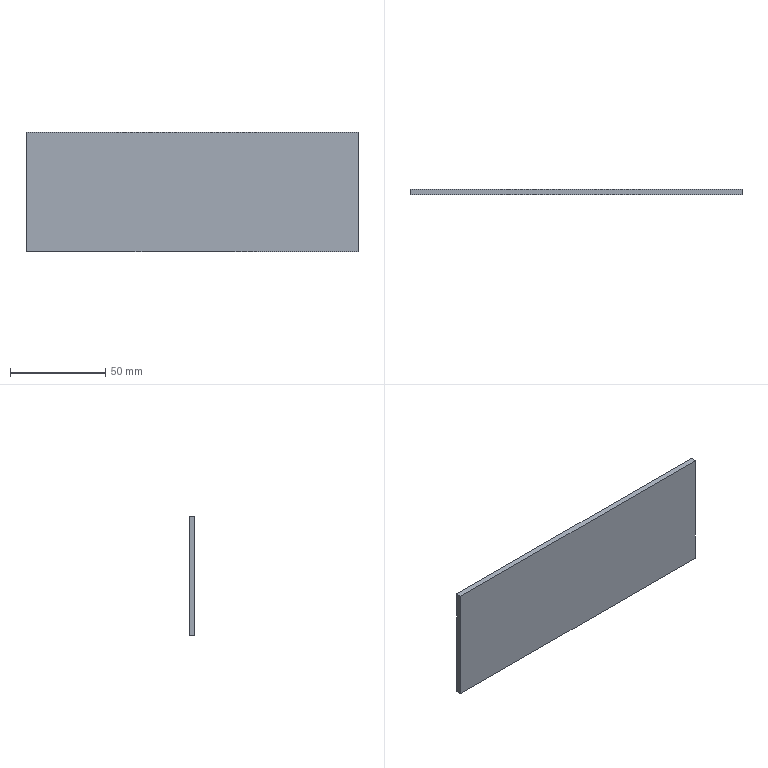Part | SolidWorks | features BaseBody 1 | 1 solid | 6 faces | box 174 x 3 x 62.5 mm | volume 32625 mm3 | plane 6
STEP:
#1=CARTESIAN_POINT('',(87.,-59.7,63.5));
#2=VERTEX_POINT('',#1);
#3=CARTESIAN_POINT('',(-87.,-59.7,63.5));
#4=VERTEX_POINT('',#3);
#5=CARTESIAN_POINT('',(0.,-59.7,63.5));
#6=DIRECTION('',(-1.,0.,0.));
#7=VECTOR('',#6,1000.);
#8=LINE('',#5,#7);
#9=EDGE_CURVE('',#2,#4,#8,.T.);
#10=ORIENTED_EDGE('',*,*,#9,.F.);
#11=CARTESIAN_POINT('',(87.,-59.7,1.));
#12=VERTEX_POINT('',#11);
#13=CARTESIAN_POINT('',(87.,-59.7,32.25));
#14=DIRECTION('',(0.,0.,1.));
#15=VECTOR('',#14,1000.);
#16=LINE('',#13,#15);
#17=EDGE_CURVE('',#12,#2,#16,.T.);
#18=ORIENTED_EDGE('',*,*,#17,.F.);
#19=CARTESIAN_POINT('',(-87.,-59.7,1.));
#20=VERTEX_POINT('',#19);
#21=CARTESIAN_POINT('',(0.,-59.7,1.));
#22=DIRECTION('',(1.,0.,0.));
#23=VECTOR('',#22,1000.);
#24=LINE('',#21,#23);
#25=EDGE_CURVE('',#20,#12,#24,.T.);
#26=ORIENTED_EDGE('',*,*,#25,.F.);
#27=CARTESIAN_POINT('',(-87.,-59.7,32.25));
#28=DIRECTION('',(0.,0.,-1.));
#29=VECTOR('',#28,1000.);
#30=LINE('',#27,#29);
#31=EDGE_CURVE('',#4,#20,#30,.T.);
#32=ORIENTED_EDGE('',*,*,#31,.F.);
#33=EDGE_LOOP('',(#10,#18,#26,#32));
#34=FACE_OUTER_BOUND('',#33,.T.);
#35=CARTESIAN_POINT('',(-90.48,-59.7,-0.25));
#36=DIRECTION('',(0.,-1.,0.));
#37=DIRECTION('',(1.,0.,0.));
#38=AXIS2_PLACEMENT_3D('',#35,#36,#37);
#39=PLANE('',#38);
#40=ADVANCED_FACE('',(#34),#39,.F.);
#41=CARTESIAN_POINT('',(-87.,-62.7,1.));
#42=VERTEX_POINT('',#41);
#43=CARTESIAN_POINT('',(-87.,-62.7,63.5));
#44=VERTEX_POINT('',#43);
#45=CARTESIAN_POINT('',(-87.,-62.7,32.25));
#46=DIRECTION('',(0.,0.,1.));
#47=VECTOR('',#46,1000.);
#48=LINE('',#45,#47);
#49=EDGE_CURVE('',#42,#44,#48,.T.);
#50=ORIENTED_EDGE('',*,*,#49,.T.);
#51=CARTESIAN_POINT('',(-87.,-61.2,63.5));
#52=DIRECTION('',(0.,1.,0.));
#53=VECTOR('',#52,1000.);
#54=LINE('',#51,#53);
#55=EDGE_CURVE('',#44,#4,#54,.T.);
#56=ORIENTED_EDGE('',*,*,#55,.T.);
#57=ORIENTED_EDGE('',*,*,#31,.T.);
#58=CARTESIAN_POINT('',(-87.,-61.2,1.));
#59=DIRECTION('',(0.,-1.,0.));
#60=VECTOR('',#59,1000.);
#61=LINE('',#58,#60);
#62=EDGE_CURVE('',#20,#42,#61,.T.);
#63=ORIENTED_EDGE('',*,*,#62,.T.);
#64=EDGE_LOOP('',(#50,#56,#57,#63));
#65=FACE_OUTER_BOUND('',#64,.T.);
#66=CARTESIAN_POINT('',(-87.,-59.478,64.75));
#67=DIRECTION('',(-1.,0.,0.));
#68=DIRECTION('',(0.,0.,-1.));
#69=AXIS2_PLACEMENT_3D('',#66,#67,#68);
#70=PLANE('',#69);
#71=ADVANCED_FACE('',(#65),#70,.T.);
#72=CARTESIAN_POINT('',(87.,-62.7,63.5));
#73=VERTEX_POINT('',#72);
#74=CARTESIAN_POINT('',(0.,-62.7,63.5));
#75=DIRECTION('',(1.,0.,0.));
#76=VECTOR('',#75,1000.);
#77=LINE('',#74,#76);
#78=EDGE_CURVE('',#44,#73,#77,.T.);
#79=ORIENTED_EDGE('',*,*,#78,.T.);
#80=CARTESIAN_POINT('',(87.,-61.2,63.5));
#81=DIRECTION('',(0.,1.,0.));
#82=VECTOR('',#81,1000.);
#83=LINE('',#80,#82);
#84=EDGE_CURVE('',#73,#2,#83,.T.);
#85=ORIENTED_EDGE('',*,*,#84,.T.);
#86=ORIENTED_EDGE('',*,*,#9,.T.);
#87=ORIENTED_EDGE('',*,*,#55,.F.);
#88=EDGE_LOOP('',(#79,#85,#86,#87));
#89=FACE_OUTER_BOUND('',#88,.T.);
#90=CARTESIAN_POINT('',(90.48,-59.478,63.5));
#91=DIRECTION('',(0.,0.,1.));
#92=DIRECTION('',(-1.,0.,0.));
#93=AXIS2_PLACEMENT_3D('',#90,#91,#92);
#94=PLANE('',#93);
#95=ADVANCED_FACE('',(#89),#94,.T.);
#96=CARTESIAN_POINT('',(87.,-62.7,1.));
#97=VERTEX_POINT('',#96);
#98=CARTESIAN_POINT('',(87.,-62.7,32.25));
#99=DIRECTION('',(0.,0.,-1.));
#100=VECTOR('',#99,1000.);
#101=LINE('',#98,#100);
#102=EDGE_CURVE('',#73,#97,#101,.T.);
#103=ORIENTED_EDGE('',*,*,#102,.T.);
#104=CARTESIAN_POINT('',(87.,-61.2,1.));
#105=DIRECTION('',(0.,1.,0.));
#106=VECTOR('',#105,1000.);
#107=LINE('',#104,#106);
#108=EDGE_CURVE('',#97,#12,#107,.T.);
#109=ORIENTED_EDGE('',*,*,#108,.T.);
#110=ORIENTED_EDGE('',*,*,#17,.T.);
#111=ORIENTED_EDGE('',*,*,#84,.F.);
#112=EDGE_LOOP('',(#103,#109,#110,#111));
#113=FACE_OUTER_BOUND('',#112,.T.);
#114=CARTESIAN_POINT('',(87.,-59.478,-0.25));
#115=DIRECTION('',(1.,0.,0.));
#116=DIRECTION('',(0.,0.,1.));
#117=AXIS2_PLACEMENT_3D('',#114,#115,#116);
#118=PLANE('',#117);
#119=ADVANCED_FACE('',(#113),#118,.T.);
#120=CARTESIAN_POINT('',(0.,-62.7,1.));
#121=DIRECTION('',(-1.,0.,0.));
#122=VECTOR('',#121,1000.);
#123=LINE('',#120,#122);
#124=EDGE_CURVE('',#97,#42,#123,.T.);
#125=ORIENTED_EDGE('',*,*,#124,.T.);
#126=ORIENTED_EDGE('',*,*,#62,.F.);
#127=ORIENTED_EDGE('',*,*,#25,.T.);
#128=ORIENTED_EDGE('',*,*,#108,.F.);
#129=EDGE_LOOP('',(#125,#126,#127,#128));
#130=FACE_OUTER_BOUND('',#129,.T.);
#131=CARTESIAN_POINT('',(-90.48,-59.478,1.));
#132=DIRECTION('',(0.,0.,-1.));
#133=DIRECTION('',(1.,0.,0.));
#134=AXIS2_PLACEMENT_3D('',#131,#132,#133);
#135=PLANE('',#134);
#136=ADVANCED_FACE('',(#130),#135,.T.);
#137=ORIENTED_EDGE('',*,*,#78,.F.);
#138=ORIENTED_EDGE('',*,*,#49,.F.);
#139=ORIENTED_EDGE('',*,*,#124,.F.);
#140=ORIENTED_EDGE('',*,*,#102,.F.);
#141=EDGE_LOOP('',(#137,#138,#139,#140));
#142=FACE_OUTER_BOUND('',#141,.T.);
#143=CARTESIAN_POINT('',(-90.48,-62.7,-0.25));
#144=DIRECTION('',(0.,-1.,0.));
#145=DIRECTION('',(1.,0.,0.));
#146=AXIS2_PLACEMENT_3D('',#143,#144,#145);
#147=PLANE('',#146);
#148=ADVANCED_FACE('',(#142),#147,.T.);
#149=CLOSED_SHELL('',(#40,#71,#95,#119,#136,#148));
#150=MANIFOLD_SOLID_BREP('',#149);
#151=CARTESIAN_POINT('',(0.,0.,0.));
#152=DIRECTION('',(0.,0.,1.));
#153=DIRECTION('',(1.,0.,0.));
#154=AXIS2_PLACEMENT_3D('',#151,#152,#153);
#155=(LENGTH_UNIT()NAMED_UNIT(*)SI_UNIT(.MILLI.,.METRE.));
#156=UNCERTAINTY_MEASURE_WITH_UNIT(LENGTH_MEASURE(0.00001),#155,'','');
#157=(NAMED_UNIT(*)PLANE_ANGLE_UNIT()SI_UNIT($,.RADIAN.));
#158=(NAMED_UNIT(*)SI_UNIT($,.STERADIAN.)SOLID_ANGLE_UNIT());
#159=(GEOMETRIC_REPRESENTATION_CONTEXT(3)GLOBAL_UNCERTAINTY_ASSIGNED_CONTEXT((#156))GLOBAL_UNIT_ASSIGNED_CONTEXT((#155,#157,#158))REPRESENTATION_CONTEXT('',''));
#160=ADVANCED_BREP_SHAPE_REPRESENTATION('',(#150,#154),#159);